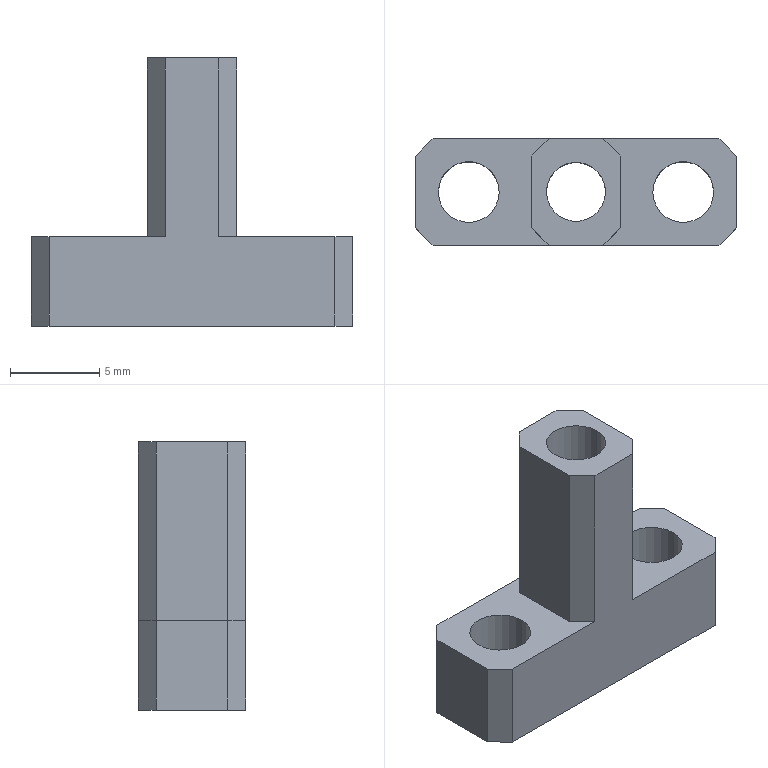Part | SolidWorks | features Chamfer 2, HoleWzd 2, Extrusion 1, ICE 1 | 1 solid | 24 faces | box 18 x 6 x 15 mm | volume 590.913 mm3 | plane 18 | cylinder 6 | commonest cylinder face diameters 3.4 x4 3.3 x2
STEP:
#1=CARTESIAN_POINT('',(1.65,0.,7.5));
#2=VERTEX_POINT('',#1);
#3=CARTESIAN_POINT('',(-1.65,0.,7.5));
#4=VERTEX_POINT('',#3);
#5=CARTESIAN_POINT('',(0.,0.,7.5));
#6=DIRECTION('',(0.,0.,-1.));
#7=DIRECTION('',(-1.,0.,0.));
#8=AXIS2_PLACEMENT_3D('',#5,#6,#7);
#9=CIRCLE('',#8,1.65);
#10=EDGE_CURVE('',#2,#4,#9,.T.);
#11=ORIENTED_EDGE('',*,*,#10,.F.);
#12=CARTESIAN_POINT('',(1.65,0.,-7.5));
#13=VERTEX_POINT('',#12);
#14=CARTESIAN_POINT('',(1.65,0.,-7.5));
#15=DIRECTION('',(0.,0.,-1.));
#16=VECTOR('',#15,1000.);
#17=LINE('',#14,#16);
#18=EDGE_CURVE('',#2,#13,#17,.T.);
#19=ORIENTED_EDGE('',*,*,#18,.T.);
#20=CARTESIAN_POINT('',(-1.65,0.,-7.5));
#21=VERTEX_POINT('',#20);
#22=CARTESIAN_POINT('',(0.,0.,-7.5));
#23=DIRECTION('',(0.,0.,-1.));
#24=DIRECTION('',(-1.,0.,0.));
#25=AXIS2_PLACEMENT_3D('',#22,#23,#24);
#26=CIRCLE('',#25,1.65);
#27=EDGE_CURVE('',#13,#21,#26,.T.);
#28=ORIENTED_EDGE('',*,*,#27,.T.);
#29=CARTESIAN_POINT('',(-1.65,0.,-7.5));
#30=DIRECTION('',(0.,0.,-1.));
#31=VECTOR('',#30,1000.);
#32=LINE('',#29,#31);
#33=EDGE_CURVE('',#4,#21,#32,.T.);
#34=ORIENTED_EDGE('',*,*,#33,.F.);
#35=EDGE_LOOP('',(#11,#19,#28,#34));
#36=FACE_OUTER_BOUND('',#35,.T.);
#37=CARTESIAN_POINT('',(0.,0.,-7.5));
#38=DIRECTION('',(0.,0.,-1.));
#39=DIRECTION('',(-1.,0.,0.));
#40=AXIS2_PLACEMENT_3D('',#37,#38,#39);
#41=CYLINDRICAL_SURFACE('',#40,1.65);
#42=ADVANCED_FACE('',(#36),#41,.F.);
#43=CARTESIAN_POINT('',(4.3,0.,-2.5));
#44=VERTEX_POINT('',#43);
#45=CARTESIAN_POINT('',(7.7,0.,-2.5));
#46=VERTEX_POINT('',#45);
#47=CARTESIAN_POINT('',(6.,0.,-2.5));
#48=DIRECTION('',(0.,0.,1.));
#49=DIRECTION('',(-1.,0.,0.));
#50=AXIS2_PLACEMENT_3D('',#47,#48,#49);
#51=CIRCLE('',#50,1.7);
#52=EDGE_CURVE('',#44,#46,#51,.T.);
#53=ORIENTED_EDGE('',*,*,#52,.T.);
#54=CARTESIAN_POINT('',(7.7,0.,-7.5));
#55=VERTEX_POINT('',#54);
#56=CARTESIAN_POINT('',(7.7,0.,-7.5));
#57=DIRECTION('',(0.,0.,-1.));
#58=VECTOR('',#57,1000.);
#59=LINE('',#56,#58);
#60=EDGE_CURVE('',#46,#55,#59,.T.);
#61=ORIENTED_EDGE('',*,*,#60,.T.);
#62=CARTESIAN_POINT('',(4.3,0.,-7.5));
#63=VERTEX_POINT('',#62);
#64=CARTESIAN_POINT('',(6.,0.,-7.5));
#65=DIRECTION('',(0.,0.,-1.));
#66=DIRECTION('',(-1.,0.,0.));
#67=AXIS2_PLACEMENT_3D('',#64,#65,#66);
#68=CIRCLE('',#67,1.7);
#69=EDGE_CURVE('',#55,#63,#68,.T.);
#70=ORIENTED_EDGE('',*,*,#69,.T.);
#71=CARTESIAN_POINT('',(4.3,0.,-7.5));
#72=DIRECTION('',(0.,0.,-1.));
#73=VECTOR('',#72,1000.);
#74=LINE('',#71,#73);
#75=EDGE_CURVE('',#44,#63,#74,.T.);
#76=ORIENTED_EDGE('',*,*,#75,.F.);
#77=EDGE_LOOP('',(#53,#61,#70,#76));
#78=FACE_OUTER_BOUND('',#77,.T.);
#79=CARTESIAN_POINT('',(6.,0.,-7.5));
#80=DIRECTION('',(0.,0.,-1.));
#81=DIRECTION('',(-1.,0.,0.));
#82=AXIS2_PLACEMENT_3D('',#79,#80,#81);
#83=CYLINDRICAL_SURFACE('',#82,1.7);
#84=ADVANCED_FACE('',(#78),#83,.F.);
#85=CARTESIAN_POINT('',(-7.7,0.,-2.5));
#86=VERTEX_POINT('',#85);
#87=CARTESIAN_POINT('',(-4.3,0.,-2.5));
#88=VERTEX_POINT('',#87);
#89=CARTESIAN_POINT('',(-6.,0.,-2.5));
#90=DIRECTION('',(0.,0.,1.));
#91=DIRECTION('',(-1.,0.,0.));
#92=AXIS2_PLACEMENT_3D('',#89,#90,#91);
#93=CIRCLE('',#92,1.7);
#94=EDGE_CURVE('',#86,#88,#93,.T.);
#95=ORIENTED_EDGE('',*,*,#94,.T.);
#96=CARTESIAN_POINT('',(-4.3,0.,-7.5));
#97=VERTEX_POINT('',#96);
#98=CARTESIAN_POINT('',(-4.3,0.,-7.5));
#99=DIRECTION('',(0.,0.,-1.));
#100=VECTOR('',#99,1000.);
#101=LINE('',#98,#100);
#102=EDGE_CURVE('',#88,#97,#101,.T.);
#103=ORIENTED_EDGE('',*,*,#102,.T.);
#104=CARTESIAN_POINT('',(-7.7,0.,-7.5));
#105=VERTEX_POINT('',#104);
#106=CARTESIAN_POINT('',(-6.,0.,-7.5));
#107=DIRECTION('',(0.,0.,-1.));
#108=DIRECTION('',(-1.,0.,0.));
#109=AXIS2_PLACEMENT_3D('',#106,#107,#108);
#110=CIRCLE('',#109,1.7);
#111=EDGE_CURVE('',#97,#105,#110,.T.);
#112=ORIENTED_EDGE('',*,*,#111,.T.);
#113=CARTESIAN_POINT('',(-7.7,0.,-7.5));
#114=DIRECTION('',(0.,0.,-1.));
#115=VECTOR('',#114,1000.);
#116=LINE('',#113,#115);
#117=EDGE_CURVE('',#86,#105,#116,.T.);
#118=ORIENTED_EDGE('',*,*,#117,.F.);
#119=EDGE_LOOP('',(#95,#103,#112,#118));
#120=FACE_OUTER_BOUND('',#119,.T.);
#121=CARTESIAN_POINT('',(-6.,0.,-7.5));
#122=DIRECTION('',(0.,0.,-1.));
#123=DIRECTION('',(-1.,0.,0.));
#124=AXIS2_PLACEMENT_3D('',#121,#122,#123);
#125=CYLINDRICAL_SURFACE('',#124,1.7);
#126=ADVANCED_FACE('',(#120),#125,.F.);
#127=CARTESIAN_POINT('',(0.,0.,7.5));
#128=DIRECTION('',(0.,0.,-1.));
#129=DIRECTION('',(-1.,0.,0.));
#130=AXIS2_PLACEMENT_3D('',#127,#128,#129);
#131=CIRCLE('',#130,1.65);
#132=EDGE_CURVE('',#4,#2,#131,.T.);
#133=ORIENTED_EDGE('',*,*,#132,.T.);
#134=ORIENTED_EDGE('',*,*,#10,.T.);
#135=EDGE_LOOP('',(#133,#134));
#136=FACE_BOUND('',#135,.T.);
#137=CARTESIAN_POINT('',(-1.5,3.,7.5));
#138=VERTEX_POINT('',#137);
#139=CARTESIAN_POINT('',(1.5,3.,7.5));
#140=VERTEX_POINT('',#139);
#141=CARTESIAN_POINT('',(0.,3.,7.5));
#142=DIRECTION('',(1.,0.,0.));
#143=VECTOR('',#142,1000.);
#144=LINE('',#141,#143);
#145=EDGE_CURVE('',#138,#140,#144,.T.);
#146=ORIENTED_EDGE('',*,*,#145,.F.);
#147=CARTESIAN_POINT('',(-2.5,2.,7.5));
#148=VERTEX_POINT('',#147);
#149=CARTESIAN_POINT('',(-1.5,3.,7.5));
#150=DIRECTION('',(-0.7071,-0.7071,0.));
#151=VECTOR('',#150,1000.);
#152=LINE('',#149,#151);
#153=EDGE_CURVE('',#138,#148,#152,.T.);
#154=ORIENTED_EDGE('',*,*,#153,.T.);
#155=CARTESIAN_POINT('',(-2.5,-2.,7.5));
#156=VERTEX_POINT('',#155);
#157=CARTESIAN_POINT('',(-2.5,3.,7.5));
#158=DIRECTION('',(0.,-1.,0.));
#159=VECTOR('',#158,1000.);
#160=LINE('',#157,#159);
#161=EDGE_CURVE('',#148,#156,#160,.T.);
#162=ORIENTED_EDGE('',*,*,#161,.T.);
#163=CARTESIAN_POINT('',(-1.5,-3.,7.5));
#164=VERTEX_POINT('',#163);
#165=CARTESIAN_POINT('',(-2.5,-2.,7.5));
#166=DIRECTION('',(0.7071,-0.7071,0.));
#167=VECTOR('',#166,1000.);
#168=LINE('',#165,#167);
#169=EDGE_CURVE('',#156,#164,#168,.T.);
#170=ORIENTED_EDGE('',*,*,#169,.T.);
#171=CARTESIAN_POINT('',(1.5,-3.,7.5));
#172=VERTEX_POINT('',#171);
#173=CARTESIAN_POINT('',(0.,-3.,7.5));
#174=DIRECTION('',(1.,0.,0.));
#175=VECTOR('',#174,1000.);
#176=LINE('',#173,#175);
#177=EDGE_CURVE('',#164,#172,#176,.T.);
#178=ORIENTED_EDGE('',*,*,#177,.T.);
#179=CARTESIAN_POINT('',(2.5,-2.,7.5));
#180=VERTEX_POINT('',#179);
#181=CARTESIAN_POINT('',(2.5,-2.,7.5));
#182=DIRECTION('',(0.7071,0.7071,0.));
#183=VECTOR('',#182,1000.);
#184=LINE('',#181,#183);
#185=EDGE_CURVE('',#172,#180,#184,.T.);
#186=ORIENTED_EDGE('',*,*,#185,.T.);
#187=CARTESIAN_POINT('',(2.5,2.,7.5));
#188=VERTEX_POINT('',#187);
#189=CARTESIAN_POINT('',(2.5,3.,7.5));
#190=DIRECTION('',(0.,-1.,0.));
#191=VECTOR('',#190,1000.);
#192=LINE('',#189,#191);
#193=EDGE_CURVE('',#188,#180,#192,.T.);
#194=ORIENTED_EDGE('',*,*,#193,.F.);
#195=CARTESIAN_POINT('',(1.5,3.,7.5));
#196=DIRECTION('',(-0.7071,0.7071,0.));
#197=VECTOR('',#196,1000.);
#198=LINE('',#195,#197);
#199=EDGE_CURVE('',#188,#140,#198,.T.);
#200=ORIENTED_EDGE('',*,*,#199,.T.);
#201=EDGE_LOOP('',(#146,#154,#162,#170,#178,#186,#194,#200));
#202=FACE_OUTER_BOUND('',#201,.T.);
#203=CARTESIAN_POINT('',(0.,3.,7.5));
#204=DIRECTION('',(0.,0.,-1.));
#205=DIRECTION('',(-1.,0.,0.));
#206=AXIS2_PLACEMENT_3D('',#203,#204,#205);
#207=PLANE('',#206);
#208=ADVANCED_FACE('',(#136,#202),#207,.F.);
#209=CARTESIAN_POINT('',(9.,2.,-7.5));
#210=VERTEX_POINT('',#209);
#211=CARTESIAN_POINT('',(9.,2.,-2.5));
#212=VERTEX_POINT('',#211);
#213=CARTESIAN_POINT('',(9.,2.,7.5));
#214=DIRECTION('',(0.,0.,1.));
#215=VECTOR('',#214,1000.);
#216=LINE('',#213,#215);
#217=EDGE_CURVE('',#210,#212,#216,.T.);
#218=ORIENTED_EDGE('',*,*,#217,.T.);
#219=CARTESIAN_POINT('',(9.,-2.,-2.5));
#220=VERTEX_POINT('',#219);
#221=CARTESIAN_POINT('',(9.,3.,-2.5));
#222=DIRECTION('',(0.,-1.,0.));
#223=VECTOR('',#222,1000.);
#224=LINE('',#221,#223);
#225=EDGE_CURVE('',#212,#220,#224,.T.);
#226=ORIENTED_EDGE('',*,*,#225,.T.);
#227=CARTESIAN_POINT('',(9.,-2.,-7.5));
#228=VERTEX_POINT('',#227);
#229=CARTESIAN_POINT('',(9.,-2.,0.));
#230=DIRECTION('',(0.,0.,-1.));
#231=VECTOR('',#230,1000.);
#232=LINE('',#229,#231);
#233=EDGE_CURVE('',#220,#228,#232,.T.);
#234=ORIENTED_EDGE('',*,*,#233,.T.);
#235=CARTESIAN_POINT('',(9.,3.,-7.5));
#236=DIRECTION('',(0.,-1.,0.));
#237=VECTOR('',#236,1000.);
#238=LINE('',#235,#237);
#239=EDGE_CURVE('',#210,#228,#238,.T.);
#240=ORIENTED_EDGE('',*,*,#239,.F.);
#241=EDGE_LOOP('',(#218,#226,#234,#240));
#242=FACE_OUTER_BOUND('',#241,.T.);
#243=CARTESIAN_POINT('',(9.,3.,0.));
#244=DIRECTION('',(-1.,0.,0.));
#245=DIRECTION('',(0.,0.,1.));
#246=AXIS2_PLACEMENT_3D('',#243,#244,#245);
#247=PLANE('',#246);
#248=ADVANCED_FACE('',(#242),#247,.F.);
#249=CARTESIAN_POINT('',(0.,0.,-7.5));
#250=DIRECTION('',(0.,0.,-1.));
#251=DIRECTION('',(-1.,0.,0.));
#252=AXIS2_PLACEMENT_3D('',#249,#250,#251);
#253=CIRCLE('',#252,1.65);
#254=EDGE_CURVE('',#21,#13,#253,.T.);
#255=ORIENTED_EDGE('',*,*,#254,.F.);
#256=ORIENTED_EDGE('',*,*,#27,.F.);
#257=EDGE_LOOP('',(#255,#256));
#258=FACE_BOUND('',#257,.T.);
#259=CARTESIAN_POINT('',(6.,0.,-7.5));
#260=DIRECTION('',(0.,0.,-1.));
#261=DIRECTION('',(-1.,0.,0.));
#262=AXIS2_PLACEMENT_3D('',#259,#260,#261);
#263=CIRCLE('',#262,1.7);
#264=EDGE_CURVE('',#63,#55,#263,.T.);
#265=ORIENTED_EDGE('',*,*,#264,.F.);
#266=ORIENTED_EDGE('',*,*,#69,.F.);
#267=EDGE_LOOP('',(#265,#266));
#268=FACE_BOUND('',#267,.T.);
#269=CARTESIAN_POINT('',(-6.,0.,-7.5));
#270=DIRECTION('',(0.,0.,-1.));
#271=DIRECTION('',(-1.,0.,0.));
#272=AXIS2_PLACEMENT_3D('',#269,#270,#271);
#273=CIRCLE('',#272,1.7);
#274=EDGE_CURVE('',#105,#97,#273,.T.);
#275=ORIENTED_EDGE('',*,*,#274,.F.);
#276=ORIENTED_EDGE('',*,*,#111,.F.);
#277=EDGE_LOOP('',(#275,#276));
#278=FACE_BOUND('',#277,.T.);
#279=CARTESIAN_POINT('',(-9.,2.,-7.5));
#280=VERTEX_POINT('',#279);
#281=CARTESIAN_POINT('',(-9.,-2.,-7.5));
#282=VERTEX_POINT('',#281);
#283=CARTESIAN_POINT('',(-9.,3.,-7.5));
#284=DIRECTION('',(0.,-1.,0.));
#285=VECTOR('',#284,1000.);
#286=LINE('',#283,#285);
#287=EDGE_CURVE('',#280,#282,#286,.T.);
#288=ORIENTED_EDGE('',*,*,#287,.F.);
#289=CARTESIAN_POINT('',(-8.,3.,-7.5));
#290=VERTEX_POINT('',#289);
#291=CARTESIAN_POINT('',(-4.,7.,-7.5));
#292=DIRECTION('',(0.7071,0.7071,0.));
#293=VECTOR('',#292,1000.);
#294=LINE('',#291,#293);
#295=EDGE_CURVE('',#280,#290,#294,.T.);
#296=ORIENTED_EDGE('',*,*,#295,.T.);
#297=CARTESIAN_POINT('',(8.,3.,-7.5));
#298=VERTEX_POINT('',#297);
#299=CARTESIAN_POINT('',(0.,3.,-7.5));
#300=DIRECTION('',(1.,0.,0.));
#301=VECTOR('',#300,1000.);
#302=LINE('',#299,#301);
#303=EDGE_CURVE('',#290,#298,#302,.T.);
#304=ORIENTED_EDGE('',*,*,#303,.T.);
#305=CARTESIAN_POINT('',(4.,7.,-7.5));
#306=DIRECTION('',(0.7071,-0.7071,0.));
#307=VECTOR('',#306,1000.);
#308=LINE('',#305,#307);
#309=EDGE_CURVE('',#298,#210,#308,.T.);
#310=ORIENTED_EDGE('',*,*,#309,.T.);
#311=ORIENTED_EDGE('',*,*,#239,.T.);
#312=CARTESIAN_POINT('',(8.,-3.,-7.5));
#313=VERTEX_POINT('',#312);
#314=CARTESIAN_POINT('',(7.,-4.,-7.5));
#315=DIRECTION('',(-0.7071,-0.7071,0.));
#316=VECTOR('',#315,1000.);
#317=LINE('',#314,#316);
#318=EDGE_CURVE('',#228,#313,#317,.T.);
#319=ORIENTED_EDGE('',*,*,#318,.T.);
#320=CARTESIAN_POINT('',(-8.,-3.,-7.5));
#321=VERTEX_POINT('',#320);
#322=CARTESIAN_POINT('',(0.,-3.,-7.5));
#323=DIRECTION('',(1.,0.,0.));
#324=VECTOR('',#323,1000.);
#325=LINE('',#322,#324);
#326=EDGE_CURVE('',#321,#313,#325,.T.);
#327=ORIENTED_EDGE('',*,*,#326,.F.);
#328=CARTESIAN_POINT('',(-7.,-4.,-7.5));
#329=DIRECTION('',(-0.7071,0.7071,0.));
#330=VECTOR('',#329,1000.);
#331=LINE('',#328,#330);
#332=EDGE_CURVE('',#321,#282,#331,.T.);
#333=ORIENTED_EDGE('',*,*,#332,.T.);
#334=EDGE_LOOP('',(#288,#296,#304,#310,#311,#319,#327,#333));
#335=FACE_OUTER_BOUND('',#334,.T.);
#336=CARTESIAN_POINT('',(0.,3.,-7.5));
#337=DIRECTION('',(0.,0.,-1.));
#338=DIRECTION('',(-1.,0.,0.));
#339=AXIS2_PLACEMENT_3D('',#336,#337,#338);
#340=PLANE('',#339);
#341=ADVANCED_FACE('',(#258,#268,#278,#335),#340,.T.);
#342=CARTESIAN_POINT('',(-9.,2.,-2.5));
#343=VERTEX_POINT('',#342);
#344=CARTESIAN_POINT('',(-9.,-2.,-2.5));
#345=VERTEX_POINT('',#344);
#346=CARTESIAN_POINT('',(-9.,3.,-2.5));
#347=DIRECTION('',(0.,-1.,0.));
#348=VECTOR('',#347,1000.);
#349=LINE('',#346,#348);
#350=EDGE_CURVE('',#343,#345,#349,.T.);
#351=ORIENTED_EDGE('',*,*,#350,.F.);
#352=CARTESIAN_POINT('',(-9.,2.,0.));
#353=DIRECTION('',(0.,0.,-1.));
#354=VECTOR('',#353,1000.);
#355=LINE('',#352,#354);
#356=EDGE_CURVE('',#343,#280,#355,.T.);
#357=ORIENTED_EDGE('',*,*,#356,.T.);
#358=ORIENTED_EDGE('',*,*,#287,.T.);
#359=CARTESIAN_POINT('',(-9.,-2.,7.5));
#360=DIRECTION('',(0.,0.,1.));
#361=VECTOR('',#360,1000.);
#362=LINE('',#359,#361);
#363=EDGE_CURVE('',#282,#345,#362,.T.);
#364=ORIENTED_EDGE('',*,*,#363,.T.);
#365=EDGE_LOOP('',(#351,#357,#358,#364));
#366=FACE_OUTER_BOUND('',#365,.T.);
#367=CARTESIAN_POINT('',(-9.,3.,0.));
#368=DIRECTION('',(-1.,0.,0.));
#369=DIRECTION('',(0.,0.,1.));
#370=AXIS2_PLACEMENT_3D('',#367,#368,#369);
#371=PLANE('',#370);
#372=ADVANCED_FACE('',(#366),#371,.T.);
#373=CARTESIAN_POINT('',(-8.,3.,-2.5));
#374=VERTEX_POINT('',#373);
#375=CARTESIAN_POINT('',(-1.5,3.,-2.5));
#376=VERTEX_POINT('',#375);
#377=CARTESIAN_POINT('',(-9.,3.,-2.5));
#378=DIRECTION('',(1.,0.,0.));
#379=VECTOR('',#378,1000.);
#380=LINE('',#377,#379);
#381=EDGE_CURVE('',#374,#376,#380,.T.);
#382=ORIENTED_EDGE('',*,*,#381,.T.);
#383=CARTESIAN_POINT('',(-1.5,3.,7.5));
#384=DIRECTION('',(0.,0.,1.));
#385=VECTOR('',#384,1000.);
#386=LINE('',#383,#385);
#387=EDGE_CURVE('',#376,#138,#386,.T.);
#388=ORIENTED_EDGE('',*,*,#387,.T.);
#389=ORIENTED_EDGE('',*,*,#145,.T.);
#390=CARTESIAN_POINT('',(1.5,3.,-2.5));
#391=VERTEX_POINT('',#390);
#392=CARTESIAN_POINT('',(1.5,3.,-2.5));
#393=DIRECTION('',(0.,0.,-1.));
#394=VECTOR('',#393,1000.);
#395=LINE('',#392,#394);
#396=EDGE_CURVE('',#140,#391,#395,.T.);
#397=ORIENTED_EDGE('',*,*,#396,.T.);
#398=CARTESIAN_POINT('',(8.,3.,-2.5));
#399=VERTEX_POINT('',#398);
#400=CARTESIAN_POINT('',(9.,3.,-2.5));
#401=DIRECTION('',(1.,0.,0.));
#402=VECTOR('',#401,1000.);
#403=LINE('',#400,#402);
#404=EDGE_CURVE('',#391,#399,#403,.T.);
#405=ORIENTED_EDGE('',*,*,#404,.T.);
#406=CARTESIAN_POINT('',(8.,3.,-7.5));
#407=DIRECTION('',(0.,0.,-1.));
#408=VECTOR('',#407,1000.);
#409=LINE('',#406,#408);
#410=EDGE_CURVE('',#399,#298,#409,.T.);
#411=ORIENTED_EDGE('',*,*,#410,.T.);
#412=ORIENTED_EDGE('',*,*,#303,.F.);
#413=CARTESIAN_POINT('',(-8.,3.,0.));
#414=DIRECTION('',(0.,0.,1.));
#415=VECTOR('',#414,1000.);
#416=LINE('',#413,#415);
#417=EDGE_CURVE('',#290,#374,#416,.T.);
#418=ORIENTED_EDGE('',*,*,#417,.T.);
#419=EDGE_LOOP('',(#382,#388,#389,#397,#405,#411,#412,#418));
#420=FACE_OUTER_BOUND('',#419,.T.);
#421=CARTESIAN_POINT('',(0.,3.,0.));
#422=DIRECTION('',(0.,1.,0.));
#423=DIRECTION('',(0.,0.,1.));
#424=AXIS2_PLACEMENT_3D('',#421,#422,#423);
#425=PLANE('',#424);
#426=ADVANCED_FACE('',(#420),#425,.T.);
#427=ORIENTED_EDGE('',*,*,#177,.F.);
#428=CARTESIAN_POINT('',(-1.5,-3.,-2.5));
#429=VERTEX_POINT('',#428);
#430=CARTESIAN_POINT('',(-1.5,-3.,0.));
#431=DIRECTION('',(0.,0.,-1.));
#432=VECTOR('',#431,1000.);
#433=LINE('',#430,#432);
#434=EDGE_CURVE('',#164,#429,#433,.T.);
#435=ORIENTED_EDGE('',*,*,#434,.T.);
#436=CARTESIAN_POINT('',(-8.,-3.,-2.5));
#437=VERTEX_POINT('',#436);
#438=CARTESIAN_POINT('',(-9.,-3.,-2.5));
#439=DIRECTION('',(1.,0.,0.));
#440=VECTOR('',#439,1000.);
#441=LINE('',#438,#440);
#442=EDGE_CURVE('',#437,#429,#441,.T.);
#443=ORIENTED_EDGE('',*,*,#442,.F.);
#444=CARTESIAN_POINT('',(-8.,-3.,-7.5));
#445=DIRECTION('',(0.,0.,-1.));
#446=VECTOR('',#445,1000.);
#447=LINE('',#444,#446);
#448=EDGE_CURVE('',#437,#321,#447,.T.);
#449=ORIENTED_EDGE('',*,*,#448,.T.);
#450=ORIENTED_EDGE('',*,*,#326,.T.);
#451=CARTESIAN_POINT('',(8.,-3.,-2.5));
#452=VERTEX_POINT('',#451);
#453=CARTESIAN_POINT('',(8.,-3.,0.));
#454=DIRECTION('',(0.,0.,1.));
#455=VECTOR('',#454,1000.);
#456=LINE('',#453,#455);
#457=EDGE_CURVE('',#313,#452,#456,.T.);
#458=ORIENTED_EDGE('',*,*,#457,.T.);
#459=CARTESIAN_POINT('',(1.5,-3.,-2.5));
#460=VERTEX_POINT('',#459);
#461=CARTESIAN_POINT('',(9.,-3.,-2.5));
#462=DIRECTION('',(1.,0.,0.));
#463=VECTOR('',#462,1000.);
#464=LINE('',#461,#463);
#465=EDGE_CURVE('',#460,#452,#464,.T.);
#466=ORIENTED_EDGE('',*,*,#465,.F.);
#467=CARTESIAN_POINT('',(1.5,-3.,0.));
#468=DIRECTION('',(0.,0.,1.));
#469=VECTOR('',#468,1000.);
#470=LINE('',#467,#469);
#471=EDGE_CURVE('',#460,#172,#470,.T.);
#472=ORIENTED_EDGE('',*,*,#471,.T.);
#473=EDGE_LOOP('',(#427,#435,#443,#449,#450,#458,#466,#472));
#474=FACE_OUTER_BOUND('',#473,.T.);
#475=CARTESIAN_POINT('',(0.,-3.,0.));
#476=DIRECTION('',(0.,1.,0.));
#477=DIRECTION('',(0.,0.,1.));
#478=AXIS2_PLACEMENT_3D('',#475,#476,#477);
#479=PLANE('',#478);
#480=ADVANCED_FACE('',(#474),#479,.F.);
#481=ORIENTED_EDGE('',*,*,#102,.F.);
#482=CARTESIAN_POINT('',(-6.,0.,-2.5));
#483=DIRECTION('',(0.,0.,1.));
#484=DIRECTION('',(-1.,0.,0.));
#485=AXIS2_PLACEMENT_3D('',#482,#483,#484);
#486=CIRCLE('',#485,1.7);
#487=EDGE_CURVE('',#88,#86,#486,.T.);
#488=ORIENTED_EDGE('',*,*,#487,.T.);
#489=ORIENTED_EDGE('',*,*,#117,.T.);
#490=ORIENTED_EDGE('',*,*,#274,.T.);
#491=EDGE_LOOP('',(#481,#488,#489,#490));
#492=FACE_OUTER_BOUND('',#491,.T.);
#493=CARTESIAN_POINT('',(-6.,0.,-7.5));
#494=DIRECTION('',(0.,0.,-1.));
#495=DIRECTION('',(-1.,0.,0.));
#496=AXIS2_PLACEMENT_3D('',#493,#494,#495);
#497=CYLINDRICAL_SURFACE('',#496,1.7);
#498=ADVANCED_FACE('',(#492),#497,.F.);
#499=ORIENTED_EDGE('',*,*,#60,.F.);
#500=CARTESIAN_POINT('',(6.,0.,-2.5));
#501=DIRECTION('',(0.,0.,1.));
#502=DIRECTION('',(-1.,0.,0.));
#503=AXIS2_PLACEMENT_3D('',#500,#501,#502);
#504=CIRCLE('',#503,1.7);
#505=EDGE_CURVE('',#46,#44,#504,.T.);
#506=ORIENTED_EDGE('',*,*,#505,.T.);
#507=ORIENTED_EDGE('',*,*,#75,.T.);
#508=ORIENTED_EDGE('',*,*,#264,.T.);
#509=EDGE_LOOP('',(#499,#506,#507,#508));
#510=FACE_OUTER_BOUND('',#509,.T.);
#511=CARTESIAN_POINT('',(6.,0.,-7.5));
#512=DIRECTION('',(0.,0.,-1.));
#513=DIRECTION('',(-1.,0.,0.));
#514=AXIS2_PLACEMENT_3D('',#511,#512,#513);
#515=CYLINDRICAL_SURFACE('',#514,1.7);
#516=ADVANCED_FACE('',(#510),#515,.F.);
#517=CARTESIAN_POINT('',(-9.,2.,-2.5));
#518=DIRECTION('',(-0.7071,-0.7071,0.));
#519=VECTOR('',#518,1000.);
#520=LINE('',#517,#519);
#521=EDGE_CURVE('',#374,#343,#520,.T.);
#522=ORIENTED_EDGE('',*,*,#521,.F.);
#523=ORIENTED_EDGE('',*,*,#417,.F.);
#524=ORIENTED_EDGE('',*,*,#295,.F.);
#525=ORIENTED_EDGE('',*,*,#356,.F.);
#526=EDGE_LOOP('',(#522,#523,#524,#525));
#527=FACE_OUTER_BOUND('',#526,.T.);
#528=CARTESIAN_POINT('',(-9.,2.,0.));
#529=DIRECTION('',(0.7071,-0.7071,0.));
#530=DIRECTION('',(0.,0.,-1.));
#531=AXIS2_PLACEMENT_3D('',#528,#529,#530);
#532=PLANE('',#531);
#533=ADVANCED_FACE('',(#527),#532,.F.);
#534=CARTESIAN_POINT('',(-8.,-3.,-2.5));
#535=DIRECTION('',(0.7071,-0.7071,0.));
#536=VECTOR('',#535,1000.);
#537=LINE('',#534,#536);
#538=EDGE_CURVE('',#345,#437,#537,.T.);
#539=ORIENTED_EDGE('',*,*,#538,.F.);
#540=ORIENTED_EDGE('',*,*,#363,.F.);
#541=ORIENTED_EDGE('',*,*,#332,.F.);
#542=ORIENTED_EDGE('',*,*,#448,.F.);
#543=EDGE_LOOP('',(#539,#540,#541,#542));
#544=FACE_OUTER_BOUND('',#543,.T.);
#545=CARTESIAN_POINT('',(-8.,-3.,0.));
#546=DIRECTION('',(-0.7071,-0.7071,0.));
#547=DIRECTION('',(0.,0.,1.));
#548=AXIS2_PLACEMENT_3D('',#545,#546,#547);
#549=PLANE('',#548);
#550=ADVANCED_FACE('',(#544),#549,.T.);
#551=CARTESIAN_POINT('',(8.,3.,-2.5));
#552=DIRECTION('',(-0.7071,0.7071,0.));
#553=VECTOR('',#552,1000.);
#554=LINE('',#551,#553);
#555=EDGE_CURVE('',#212,#399,#554,.T.);
#556=ORIENTED_EDGE('',*,*,#555,.F.);
#557=ORIENTED_EDGE('',*,*,#217,.F.);
#558=ORIENTED_EDGE('',*,*,#309,.F.);
#559=ORIENTED_EDGE('',*,*,#410,.F.);
#560=EDGE_LOOP('',(#556,#557,#558,#559));
#561=FACE_OUTER_BOUND('',#560,.T.);
#562=CARTESIAN_POINT('',(8.,3.,0.));
#563=DIRECTION('',(0.7071,0.7071,0.));
#564=DIRECTION('',(0.,0.,1.));
#565=AXIS2_PLACEMENT_3D('',#562,#563,#564);
#566=PLANE('',#565);
#567=ADVANCED_FACE('',(#561),#566,.T.);
#568=CARTESIAN_POINT('',(9.,-2.,-2.5));
#569=DIRECTION('',(0.7071,0.7071,0.));
#570=VECTOR('',#569,1000.);
#571=LINE('',#568,#570);
#572=EDGE_CURVE('',#452,#220,#571,.T.);
#573=ORIENTED_EDGE('',*,*,#572,.F.);
#574=ORIENTED_EDGE('',*,*,#457,.F.);
#575=ORIENTED_EDGE('',*,*,#318,.F.);
#576=ORIENTED_EDGE('',*,*,#233,.F.);
#577=EDGE_LOOP('',(#573,#574,#575,#576));
#578=FACE_OUTER_BOUND('',#577,.T.);
#579=CARTESIAN_POINT('',(9.,-2.,0.));
#580=DIRECTION('',(-0.7071,0.7071,0.));
#581=DIRECTION('',(0.,0.,-1.));
#582=AXIS2_PLACEMENT_3D('',#579,#580,#581);
#583=PLANE('',#582);
#584=ADVANCED_FACE('',(#578),#583,.F.);
#585=ORIENTED_EDGE('',*,*,#555,.T.);
#586=ORIENTED_EDGE('',*,*,#404,.F.);
#587=CARTESIAN_POINT('',(2.5,2.,-2.5));
#588=VERTEX_POINT('',#587);
#589=CARTESIAN_POINT('',(5.25,-0.75,-2.5));
#590=DIRECTION('',(0.7071,-0.7071,0.));
#591=VECTOR('',#590,1000.);
#592=LINE('',#589,#591);
#593=EDGE_CURVE('',#391,#588,#592,.T.);
#594=ORIENTED_EDGE('',*,*,#593,.T.);
#595=CARTESIAN_POINT('',(2.5,-2.,-2.5));
#596=VERTEX_POINT('',#595);
#597=CARTESIAN_POINT('',(2.5,3.,-2.5));
#598=DIRECTION('',(0.,-1.,0.));
#599=VECTOR('',#598,1000.);
#600=LINE('',#597,#599);
#601=EDGE_CURVE('',#588,#596,#600,.T.);
#602=ORIENTED_EDGE('',*,*,#601,.T.);
#603=CARTESIAN_POINT('',(8.25,3.75,-2.5));
#604=DIRECTION('',(-0.7071,-0.7071,0.));
#605=VECTOR('',#604,1000.);
#606=LINE('',#603,#605);
#607=EDGE_CURVE('',#596,#460,#606,.T.);
#608=ORIENTED_EDGE('',*,*,#607,.T.);
#609=ORIENTED_EDGE('',*,*,#465,.T.);
#610=ORIENTED_EDGE('',*,*,#572,.T.);
#611=ORIENTED_EDGE('',*,*,#225,.F.);
#612=EDGE_LOOP('',(#585,#586,#594,#602,#608,#609,#610,#611));
#613=FACE_OUTER_BOUND('',#612,.T.);
#614=ORIENTED_EDGE('',*,*,#52,.F.);
#615=ORIENTED_EDGE('',*,*,#505,.F.);
#616=EDGE_LOOP('',(#614,#615));
#617=FACE_BOUND('',#616,.T.);
#618=CARTESIAN_POINT('',(9.,3.,-2.5));
#619=DIRECTION('',(0.,0.,-1.));
#620=DIRECTION('',(-1.,0.,0.));
#621=AXIS2_PLACEMENT_3D('',#618,#619,#620);
#622=PLANE('',#621);
#623=ADVANCED_FACE('',(#613,#617),#622,.F.);
#624=ORIENTED_EDGE('',*,*,#601,.F.);
#625=CARTESIAN_POINT('',(2.5,2.,7.5));
#626=DIRECTION('',(0.,0.,1.));
#627=VECTOR('',#626,1000.);
#628=LINE('',#625,#627);
#629=EDGE_CURVE('',#588,#188,#628,.T.);
#630=ORIENTED_EDGE('',*,*,#629,.T.);
#631=ORIENTED_EDGE('',*,*,#193,.T.);
#632=CARTESIAN_POINT('',(2.5,-2.,7.5));
#633=DIRECTION('',(0.,0.,-1.));
#634=VECTOR('',#633,1000.);
#635=LINE('',#632,#634);
#636=EDGE_CURVE('',#180,#596,#635,.T.);
#637=ORIENTED_EDGE('',*,*,#636,.T.);
#638=EDGE_LOOP('',(#624,#630,#631,#637));
#639=FACE_OUTER_BOUND('',#638,.T.);
#640=CARTESIAN_POINT('',(2.5,3.,7.5));
#641=DIRECTION('',(-1.,0.,0.));
#642=DIRECTION('',(0.,0.,1.));
#643=AXIS2_PLACEMENT_3D('',#640,#641,#642);
#644=PLANE('',#643);
#645=ADVANCED_FACE('',(#639),#644,.F.);
#646=ORIENTED_EDGE('',*,*,#521,.T.);
#647=ORIENTED_EDGE('',*,*,#350,.T.);
#648=ORIENTED_EDGE('',*,*,#538,.T.);
#649=ORIENTED_EDGE('',*,*,#442,.T.);
#650=CARTESIAN_POINT('',(-2.5,-2.,-2.5));
#651=VERTEX_POINT('',#650);
#652=CARTESIAN_POINT('',(-8.25,3.75,-2.5));
#653=DIRECTION('',(-0.7071,0.7071,0.));
#654=VECTOR('',#653,1000.);
#655=LINE('',#652,#654);
#656=EDGE_CURVE('',#429,#651,#655,.T.);
#657=ORIENTED_EDGE('',*,*,#656,.T.);
#658=CARTESIAN_POINT('',(-2.5,2.,-2.5));
#659=VERTEX_POINT('',#658);
#660=CARTESIAN_POINT('',(-2.5,3.,-2.5));
#661=DIRECTION('',(0.,-1.,0.));
#662=VECTOR('',#661,1000.);
#663=LINE('',#660,#662);
#664=EDGE_CURVE('',#659,#651,#663,.T.);
#665=ORIENTED_EDGE('',*,*,#664,.F.);
#666=CARTESIAN_POINT('',(-5.25,-0.75,-2.5));
#667=DIRECTION('',(0.7071,0.7071,0.));
#668=VECTOR('',#667,1000.);
#669=LINE('',#666,#668);
#670=EDGE_CURVE('',#659,#376,#669,.T.);
#671=ORIENTED_EDGE('',*,*,#670,.T.);
#672=ORIENTED_EDGE('',*,*,#381,.F.);
#673=EDGE_LOOP('',(#646,#647,#648,#649,#657,#665,#671,#672));
#674=FACE_OUTER_BOUND('',#673,.T.);
#675=ORIENTED_EDGE('',*,*,#94,.F.);
#676=ORIENTED_EDGE('',*,*,#487,.F.);
#677=EDGE_LOOP('',(#675,#676));
#678=FACE_BOUND('',#677,.T.);
#679=CARTESIAN_POINT('',(-9.,3.,-2.5));
#680=DIRECTION('',(0.,0.,-1.));
#681=DIRECTION('',(-1.,0.,0.));
#682=AXIS2_PLACEMENT_3D('',#679,#680,#681);
#683=PLANE('',#682);
#684=ADVANCED_FACE('',(#674,#678),#683,.F.);
#685=ORIENTED_EDGE('',*,*,#161,.F.);
#686=CARTESIAN_POINT('',(-2.5,2.,-2.5));
#687=DIRECTION('',(0.,0.,-1.));
#688=VECTOR('',#687,1000.);
#689=LINE('',#686,#688);
#690=EDGE_CURVE('',#148,#659,#689,.T.);
#691=ORIENTED_EDGE('',*,*,#690,.T.);
#692=ORIENTED_EDGE('',*,*,#664,.T.);
#693=CARTESIAN_POINT('',(-2.5,-2.,7.5));
#694=DIRECTION('',(0.,0.,1.));
#695=VECTOR('',#694,1000.);
#696=LINE('',#693,#695);
#697=EDGE_CURVE('',#651,#156,#696,.T.);
#698=ORIENTED_EDGE('',*,*,#697,.T.);
#699=EDGE_LOOP('',(#685,#691,#692,#698));
#700=FACE_OUTER_BOUND('',#699,.T.);
#701=CARTESIAN_POINT('',(-2.5,3.,7.5));
#702=DIRECTION('',(1.,0.,0.));
#703=DIRECTION('',(0.,0.,-1.));
#704=AXIS2_PLACEMENT_3D('',#701,#702,#703);
#705=PLANE('',#704);
#706=ADVANCED_FACE('',(#700),#705,.F.);
#707=ORIENTED_EDGE('',*,*,#18,.F.);
#708=ORIENTED_EDGE('',*,*,#132,.F.);
#709=ORIENTED_EDGE('',*,*,#33,.T.);
#710=ORIENTED_EDGE('',*,*,#254,.T.);
#711=EDGE_LOOP('',(#707,#708,#709,#710));
#712=FACE_OUTER_BOUND('',#711,.T.);
#713=CARTESIAN_POINT('',(0.,0.,-7.5));
#714=DIRECTION('',(0.,0.,-1.));
#715=DIRECTION('',(-1.,0.,0.));
#716=AXIS2_PLACEMENT_3D('',#713,#714,#715);
#717=CYLINDRICAL_SURFACE('',#716,1.65);
#718=ADVANCED_FACE('',(#712),#717,.F.);
#719=ORIENTED_EDGE('',*,*,#670,.F.);
#720=ORIENTED_EDGE('',*,*,#690,.F.);
#721=ORIENTED_EDGE('',*,*,#153,.F.);
#722=ORIENTED_EDGE('',*,*,#387,.F.);
#723=EDGE_LOOP('',(#719,#720,#721,#722));
#724=FACE_OUTER_BOUND('',#723,.T.);
#725=CARTESIAN_POINT('',(-1.5,3.,0.));
#726=DIRECTION('',(-0.7071,0.7071,0.));
#727=DIRECTION('',(0.,0.,-1.));
#728=AXIS2_PLACEMENT_3D('',#725,#726,#727);
#729=PLANE('',#728);
#730=ADVANCED_FACE('',(#724),#729,.T.);
#731=ORIENTED_EDGE('',*,*,#656,.F.);
#732=ORIENTED_EDGE('',*,*,#434,.F.);
#733=ORIENTED_EDGE('',*,*,#169,.F.);
#734=ORIENTED_EDGE('',*,*,#697,.F.);
#735=EDGE_LOOP('',(#731,#732,#733,#734));
#736=FACE_OUTER_BOUND('',#735,.T.);
#737=CARTESIAN_POINT('',(-2.5,-2.,7.5));
#738=DIRECTION('',(0.7071,0.7071,0.));
#739=DIRECTION('',(0.,0.,1.));
#740=AXIS2_PLACEMENT_3D('',#737,#738,#739);
#741=PLANE('',#740);
#742=ADVANCED_FACE('',(#736),#741,.F.);
#743=ORIENTED_EDGE('',*,*,#199,.F.);
#744=ORIENTED_EDGE('',*,*,#629,.F.);
#745=ORIENTED_EDGE('',*,*,#593,.F.);
#746=ORIENTED_EDGE('',*,*,#396,.F.);
#747=EDGE_LOOP('',(#743,#744,#745,#746));
#748=FACE_OUTER_BOUND('',#747,.T.);
#749=CARTESIAN_POINT('',(1.5,3.,0.));
#750=DIRECTION('',(0.7071,0.7071,0.));
#751=DIRECTION('',(0.,0.,1.));
#752=AXIS2_PLACEMENT_3D('',#749,#750,#751);
#753=PLANE('',#752);
#754=ADVANCED_FACE('',(#748),#753,.T.);
#755=ORIENTED_EDGE('',*,*,#185,.F.);
#756=ORIENTED_EDGE('',*,*,#471,.F.);
#757=ORIENTED_EDGE('',*,*,#607,.F.);
#758=ORIENTED_EDGE('',*,*,#636,.F.);
#759=EDGE_LOOP('',(#755,#756,#757,#758));
#760=FACE_OUTER_BOUND('',#759,.T.);
#761=CARTESIAN_POINT('',(2.5,-2.,7.5));
#762=DIRECTION('',(-0.7071,0.7071,0.));
#763=DIRECTION('',(0.,0.,-1.));
#764=AXIS2_PLACEMENT_3D('',#761,#762,#763);
#765=PLANE('',#764);
#766=ADVANCED_FACE('',(#760),#765,.F.);
#767=CLOSED_SHELL('',(#42,#84,#126,#208,#248,#341,#372,#426,#480,#498,#516,#533,#550,#567,#584,#623,#645,#684,#706,#718,#730,#742,#754,#766));
#768=MANIFOLD_SOLID_BREP('',#767);
#769=CARTESIAN_POINT('',(0.,0.,0.));
#770=DIRECTION('',(0.,0.,1.));
#771=DIRECTION('',(1.,0.,0.));
#772=AXIS2_PLACEMENT_3D('',#769,#770,#771);
#773=(LENGTH_UNIT()NAMED_UNIT(*)SI_UNIT(.MILLI.,.METRE.));
#774=UNCERTAINTY_MEASURE_WITH_UNIT(LENGTH_MEASURE(0.00001),#773,'','');
#775=(NAMED_UNIT(*)PLANE_ANGLE_UNIT()SI_UNIT($,.RADIAN.));
#776=(NAMED_UNIT(*)SI_UNIT($,.STERADIAN.)SOLID_ANGLE_UNIT());
#777=(GEOMETRIC_REPRESENTATION_CONTEXT(3)GLOBAL_UNCERTAINTY_ASSIGNED_CONTEXT((#774))GLOBAL_UNIT_ASSIGNED_CONTEXT((#773,#775,#776))REPRESENTATION_CONTEXT('',''));
#778=ADVANCED_BREP_SHAPE_REPRESENTATION('',(#768,#772),#777);